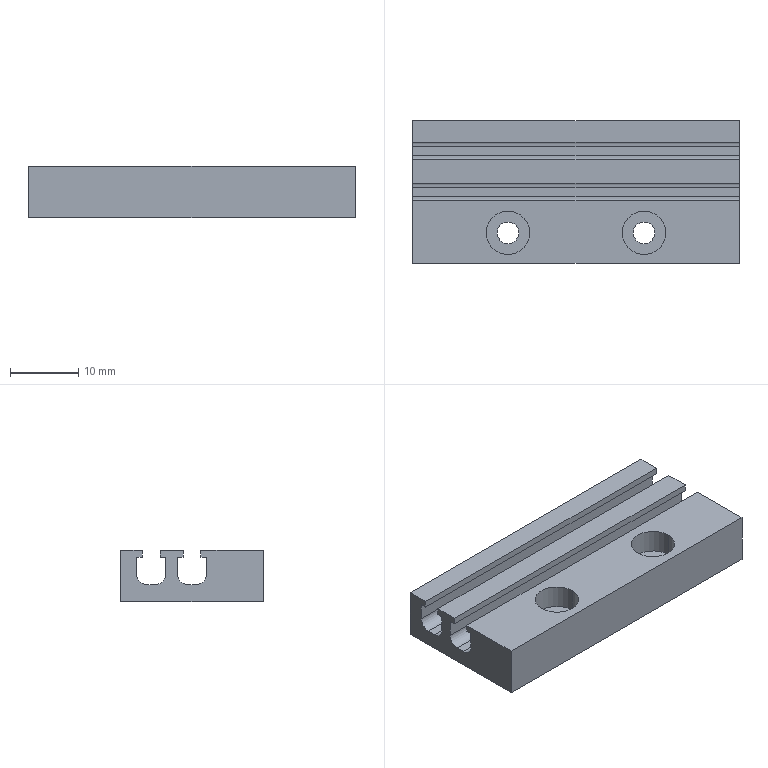Part | NX | 1 solid | 36 faces | box 48 x 21 x 7.5 mm | volume 5462 mm3 | plane 24 | cylinder 12 | commonest cylinder face diameters 3 x4 3.2 x4 6.4 x4
STEP:
#1=CARTESIAN_POINT('',(126.,-1.,-7.5));
#2=VERTEX_POINT('',#1);
#3=CARTESIAN_POINT('',(126.,-1.,0.));
#4=VERTEX_POINT('',#3);
#5=CARTESIAN_POINT('',(126.,-1.,0.));
#6=DIRECTION('',(0.,0.,1.));
#7=VECTOR('',#6,1000.);
#8=LINE('',#5,#7);
#9=EDGE_CURVE('',#2,#4,#8,.T.);
#10=ORIENTED_EDGE('',*,*,#9,.F.);
#11=CARTESIAN_POINT('',(126.,20.,-7.5));
#12=VERTEX_POINT('',#11);
#13=CARTESIAN_POINT('',(126.,0.,-7.5));
#14=DIRECTION('',(0.,1.,0.));
#15=VECTOR('',#14,1000.);
#16=LINE('',#13,#15);
#17=EDGE_CURVE('',#2,#12,#16,.T.);
#18=ORIENTED_EDGE('',*,*,#17,.T.);
#19=CARTESIAN_POINT('',(126.,20.,0.));
#20=VERTEX_POINT('',#19);
#21=CARTESIAN_POINT('',(126.,20.,0.));
#22=DIRECTION('',(0.,0.,1.));
#23=VECTOR('',#22,1000.);
#24=LINE('',#21,#23);
#25=EDGE_CURVE('',#12,#20,#24,.T.);
#26=ORIENTED_EDGE('',*,*,#25,.T.);
#27=CARTESIAN_POINT('',(126.,16.8,0.));
#28=VERTEX_POINT('',#27);
#29=CARTESIAN_POINT('',(126.,0.,0.));
#30=DIRECTION('',(0.,-1.,0.));
#31=VECTOR('',#30,1000.);
#32=LINE('',#29,#31);
#33=EDGE_CURVE('',#20,#28,#32,.T.);
#34=ORIENTED_EDGE('',*,*,#33,.T.);
#35=CARTESIAN_POINT('',(126.,16.8,-1.));
#36=VERTEX_POINT('',#35);
#37=CARTESIAN_POINT('',(126.,16.8,0.));
#38=DIRECTION('',(0.,0.,-1.));
#39=VECTOR('',#38,1000.);
#40=LINE('',#37,#39);
#41=EDGE_CURVE('',#28,#36,#40,.T.);
#42=ORIENTED_EDGE('',*,*,#41,.T.);
#43=CARTESIAN_POINT('',(126.,17.65,-1.));
#44=VERTEX_POINT('',#43);
#45=CARTESIAN_POINT('',(126.,0.,-1.));
#46=DIRECTION('',(0.,1.,0.));
#47=VECTOR('',#46,1000.);
#48=LINE('',#45,#47);
#49=EDGE_CURVE('',#36,#44,#48,.T.);
#50=ORIENTED_EDGE('',*,*,#49,.T.);
#51=CARTESIAN_POINT('',(126.,17.65,-3.5));
#52=VERTEX_POINT('',#51);
#53=CARTESIAN_POINT('',(126.,17.65,0.));
#54=DIRECTION('',(0.,0.,-1.));
#55=VECTOR('',#54,1000.);
#56=LINE('',#53,#55);
#57=EDGE_CURVE('',#44,#52,#56,.T.);
#58=ORIENTED_EDGE('',*,*,#57,.T.);
#59=CARTESIAN_POINT('',(126.,16.15,-5.));
#60=VERTEX_POINT('',#59);
#61=CARTESIAN_POINT('',(126.,16.15,-3.5));
#62=DIRECTION('',(1.,0.,0.));
#63=DIRECTION('',(0.,0.,-1.));
#64=AXIS2_PLACEMENT_3D('',#61,#62,#63);
#65=CIRCLE('',#64,1.5);
#66=EDGE_CURVE('',#60,#52,#65,.T.);
#67=ORIENTED_EDGE('',*,*,#66,.F.);
#68=CARTESIAN_POINT('',(126.,14.85,-5.));
#69=VERTEX_POINT('',#68);
#70=CARTESIAN_POINT('',(126.,0.,-5.));
#71=DIRECTION('',(0.,-1.,0.));
#72=VECTOR('',#71,1000.);
#73=LINE('',#70,#72);
#74=EDGE_CURVE('',#60,#69,#73,.T.);
#75=ORIENTED_EDGE('',*,*,#74,.T.);
#76=CARTESIAN_POINT('',(126.,13.35,-3.5));
#77=VERTEX_POINT('',#76);
#78=CARTESIAN_POINT('',(126.,14.85,-3.5));
#79=DIRECTION('',(1.,0.,0.));
#80=DIRECTION('',(0.,0.,-1.));
#81=AXIS2_PLACEMENT_3D('',#78,#79,#80);
#82=CIRCLE('',#81,1.5);
#83=EDGE_CURVE('',#77,#69,#82,.T.);
#84=ORIENTED_EDGE('',*,*,#83,.F.);
#85=CARTESIAN_POINT('',(126.,13.35,-1.));
#86=VERTEX_POINT('',#85);
#87=CARTESIAN_POINT('',(126.,13.35,0.));
#88=DIRECTION('',(0.,0.,1.));
#89=VECTOR('',#88,1000.);
#90=LINE('',#87,#89);
#91=EDGE_CURVE('',#77,#86,#90,.T.);
#92=ORIENTED_EDGE('',*,*,#91,.T.);
#93=CARTESIAN_POINT('',(126.,14.2,-1.));
#94=VERTEX_POINT('',#93);
#95=CARTESIAN_POINT('',(126.,0.,-1.));
#96=DIRECTION('',(0.,1.,0.));
#97=VECTOR('',#96,1000.);
#98=LINE('',#95,#97);
#99=EDGE_CURVE('',#86,#94,#98,.T.);
#100=ORIENTED_EDGE('',*,*,#99,.T.);
#101=CARTESIAN_POINT('',(126.,14.2,0.));
#102=VERTEX_POINT('',#101);
#103=CARTESIAN_POINT('',(126.,14.2,0.));
#104=DIRECTION('',(0.,0.,1.));
#105=VECTOR('',#104,1000.);
#106=LINE('',#103,#105);
#107=EDGE_CURVE('',#94,#102,#106,.T.);
#108=ORIENTED_EDGE('',*,*,#107,.T.);
#109=CARTESIAN_POINT('',(126.,10.8,0.));
#110=VERTEX_POINT('',#109);
#111=CARTESIAN_POINT('',(126.,0.,0.));
#112=DIRECTION('',(0.,-1.,0.));
#113=VECTOR('',#112,1000.);
#114=LINE('',#111,#113);
#115=EDGE_CURVE('',#102,#110,#114,.T.);
#116=ORIENTED_EDGE('',*,*,#115,.T.);
#117=CARTESIAN_POINT('',(126.,10.8,-1.));
#118=VERTEX_POINT('',#117);
#119=CARTESIAN_POINT('',(126.,10.8,0.));
#120=DIRECTION('',(0.,0.,-1.));
#121=VECTOR('',#120,1000.);
#122=LINE('',#119,#121);
#123=EDGE_CURVE('',#110,#118,#122,.T.);
#124=ORIENTED_EDGE('',*,*,#123,.T.);
#125=CARTESIAN_POINT('',(126.,11.65,-1.));
#126=VERTEX_POINT('',#125);
#127=CARTESIAN_POINT('',(126.,0.,-1.));
#128=DIRECTION('',(0.,1.,0.));
#129=VECTOR('',#128,1000.);
#130=LINE('',#127,#129);
#131=EDGE_CURVE('',#118,#126,#130,.T.);
#132=ORIENTED_EDGE('',*,*,#131,.T.);
#133=CARTESIAN_POINT('',(126.,11.65,-3.5));
#134=VERTEX_POINT('',#133);
#135=CARTESIAN_POINT('',(126.,11.65,0.));
#136=DIRECTION('',(0.,0.,-1.));
#137=VECTOR('',#136,1000.);
#138=LINE('',#135,#137);
#139=EDGE_CURVE('',#126,#134,#138,.T.);
#140=ORIENTED_EDGE('',*,*,#139,.T.);
#141=CARTESIAN_POINT('',(126.,10.15,-5.));
#142=VERTEX_POINT('',#141);
#143=CARTESIAN_POINT('',(126.,10.15,-3.5));
#144=DIRECTION('',(1.,0.,0.));
#145=DIRECTION('',(0.,0.,-1.));
#146=AXIS2_PLACEMENT_3D('',#143,#144,#145);
#147=CIRCLE('',#146,1.5);
#148=EDGE_CURVE('',#142,#134,#147,.T.);
#149=ORIENTED_EDGE('',*,*,#148,.F.);
#150=CARTESIAN_POINT('',(126.,8.85,-5.));
#151=VERTEX_POINT('',#150);
#152=CARTESIAN_POINT('',(126.,0.,-5.));
#153=DIRECTION('',(0.,-1.,0.));
#154=VECTOR('',#153,1000.);
#155=LINE('',#152,#154);
#156=EDGE_CURVE('',#142,#151,#155,.T.);
#157=ORIENTED_EDGE('',*,*,#156,.T.);
#158=CARTESIAN_POINT('',(126.,7.35,-3.5));
#159=VERTEX_POINT('',#158);
#160=CARTESIAN_POINT('',(126.,8.85,-3.5));
#161=DIRECTION('',(1.,0.,0.));
#162=DIRECTION('',(0.,0.,-1.));
#163=AXIS2_PLACEMENT_3D('',#160,#161,#162);
#164=CIRCLE('',#163,1.5);
#165=EDGE_CURVE('',#159,#151,#164,.T.);
#166=ORIENTED_EDGE('',*,*,#165,.F.);
#167=CARTESIAN_POINT('',(126.,7.35,-1.));
#168=VERTEX_POINT('',#167);
#169=CARTESIAN_POINT('',(126.,7.35,0.));
#170=DIRECTION('',(0.,0.,1.));
#171=VECTOR('',#170,1000.);
#172=LINE('',#169,#171);
#173=EDGE_CURVE('',#159,#168,#172,.T.);
#174=ORIENTED_EDGE('',*,*,#173,.T.);
#175=CARTESIAN_POINT('',(126.,8.2,-1.));
#176=VERTEX_POINT('',#175);
#177=CARTESIAN_POINT('',(126.,0.,-1.));
#178=DIRECTION('',(0.,1.,0.));
#179=VECTOR('',#178,1000.);
#180=LINE('',#177,#179);
#181=EDGE_CURVE('',#168,#176,#180,.T.);
#182=ORIENTED_EDGE('',*,*,#181,.T.);
#183=CARTESIAN_POINT('',(126.,8.2,0.));
#184=VERTEX_POINT('',#183);
#185=CARTESIAN_POINT('',(126.,8.2,0.));
#186=DIRECTION('',(0.,0.,1.));
#187=VECTOR('',#186,1000.);
#188=LINE('',#185,#187);
#189=EDGE_CURVE('',#176,#184,#188,.T.);
#190=ORIENTED_EDGE('',*,*,#189,.T.);
#191=CARTESIAN_POINT('',(126.,0.,0.));
#192=DIRECTION('',(0.,-1.,0.));
#193=VECTOR('',#192,1000.);
#194=LINE('',#191,#193);
#195=EDGE_CURVE('',#184,#4,#194,.T.);
#196=ORIENTED_EDGE('',*,*,#195,.T.);
#197=EDGE_LOOP('',(#10,#18,#26,#34,#42,#50,#58,#67,#75,#84,#92,#100,#108,#116,#124,#132,#140,#149,#157,#166,#174,#182,#190,#196));
#198=FACE_BOUND('',#197,.T.);
#199=CARTESIAN_POINT('',(126.,0.,0.));
#200=DIRECTION('',(1.,0.,0.));
#201=DIRECTION('',(0.,1.,0.));
#202=AXIS2_PLACEMENT_3D('',#199,#200,#201);
#203=PLANE('',#202);
#204=ADVANCED_FACE('',(#198),#203,.T.);
#205=CARTESIAN_POINT('',(78.,20.,0.));
#206=VERTEX_POINT('',#205);
#207=CARTESIAN_POINT('',(0.,20.,0.));
#208=DIRECTION('',(1.,0.,0.));
#209=VECTOR('',#208,1000.);
#210=LINE('',#207,#209);
#211=EDGE_CURVE('',#206,#20,#210,.T.);
#212=ORIENTED_EDGE('',*,*,#211,.F.);
#213=CARTESIAN_POINT('',(78.,16.8,0.));
#214=VERTEX_POINT('',#213);
#215=CARTESIAN_POINT('',(78.,0.,0.));
#216=DIRECTION('',(0.,-1.,0.));
#217=VECTOR('',#216,1000.);
#218=LINE('',#215,#217);
#219=EDGE_CURVE('',#206,#214,#218,.T.);
#220=ORIENTED_EDGE('',*,*,#219,.T.);
#221=CARTESIAN_POINT('',(0.,16.8,0.));
#222=DIRECTION('',(-1.,0.,0.));
#223=VECTOR('',#222,1000.);
#224=LINE('',#221,#223);
#225=EDGE_CURVE('',#28,#214,#224,.T.);
#226=ORIENTED_EDGE('',*,*,#225,.F.);
#227=ORIENTED_EDGE('',*,*,#33,.F.);
#228=EDGE_LOOP('',(#212,#220,#226,#227));
#229=FACE_BOUND('',#228,.T.);
#230=CARTESIAN_POINT('',(122.,19.,0.));
#231=DIRECTION('',(0.,0.,-1.));
#232=DIRECTION('',(0.,-1.,0.));
#233=AXIS2_PLACEMENT_3D('',#230,#231,#232);
#234=PLANE('',#233);
#235=ADVANCED_FACE('',(#229),#234,.F.);
#236=CARTESIAN_POINT('',(78.,20.,-7.5));
#237=VERTEX_POINT('',#236);
#238=CARTESIAN_POINT('',(0.,20.,-7.5));
#239=DIRECTION('',(-1.,0.,0.));
#240=VECTOR('',#239,1000.);
#241=LINE('',#238,#240);
#242=EDGE_CURVE('',#12,#237,#241,.T.);
#243=ORIENTED_EDGE('',*,*,#242,.T.);
#244=CARTESIAN_POINT('',(78.,20.,0.));
#245=DIRECTION('',(0.,0.,1.));
#246=VECTOR('',#245,1000.);
#247=LINE('',#244,#246);
#248=EDGE_CURVE('',#237,#206,#247,.T.);
#249=ORIENTED_EDGE('',*,*,#248,.T.);
#250=ORIENTED_EDGE('',*,*,#211,.T.);
#251=ORIENTED_EDGE('',*,*,#25,.F.);
#252=EDGE_LOOP('',(#243,#249,#250,#251));
#253=FACE_BOUND('',#252,.T.);
#254=CARTESIAN_POINT('',(122.,20.,-7.5));
#255=DIRECTION('',(0.,-1.,0.));
#256=DIRECTION('',(0.,0.,-1.));
#257=AXIS2_PLACEMENT_3D('',#254,#255,#256);
#258=PLANE('',#257);
#259=ADVANCED_FACE('',(#253),#258,.F.);
#260=CARTESIAN_POINT('',(78.,-1.,0.));
#261=VERTEX_POINT('',#260);
#262=CARTESIAN_POINT('',(0.,-1.,0.));
#263=DIRECTION('',(1.,0.,0.));
#264=VECTOR('',#263,1000.);
#265=LINE('',#262,#264);
#266=EDGE_CURVE('',#261,#4,#265,.T.);
#267=ORIENTED_EDGE('',*,*,#266,.T.);
#268=ORIENTED_EDGE('',*,*,#195,.F.);
#269=CARTESIAN_POINT('',(78.,8.2,0.));
#270=VERTEX_POINT('',#269);
#271=CARTESIAN_POINT('',(0.,8.2,0.));
#272=DIRECTION('',(1.,0.,0.));
#273=VECTOR('',#272,1000.);
#274=LINE('',#271,#273);
#275=EDGE_CURVE('',#270,#184,#274,.T.);
#276=ORIENTED_EDGE('',*,*,#275,.F.);
#277=CARTESIAN_POINT('',(78.,0.,0.));
#278=DIRECTION('',(0.,1.,0.));
#279=VECTOR('',#278,1000.);
#280=LINE('',#277,#279);
#281=EDGE_CURVE('',#261,#270,#280,.T.);
#282=ORIENTED_EDGE('',*,*,#281,.F.);
#283=EDGE_LOOP('',(#267,#268,#276,#282));
#284=FACE_BOUND('',#283,.T.);
#285=CARTESIAN_POINT('',(108.8,3.5,0.));
#286=VERTEX_POINT('',#285);
#287=CARTESIAN_POINT('',(115.2,3.5,0.));
#288=VERTEX_POINT('',#287);
#289=CARTESIAN_POINT('',(112.,3.5,0.));
#290=DIRECTION('',(0.,0.,-1.));
#291=DIRECTION('',(1.,0.,0.));
#292=AXIS2_PLACEMENT_3D('',#289,#290,#291);
#293=CIRCLE('',#292,3.2);
#294=EDGE_CURVE('',#286,#288,#293,.T.);
#295=ORIENTED_EDGE('',*,*,#294,.T.);
#296=CARTESIAN_POINT('',(112.,3.5,0.));
#297=DIRECTION('',(0.,0.,-1.));
#298=DIRECTION('',(1.,0.,0.));
#299=AXIS2_PLACEMENT_3D('',#296,#297,#298);
#300=CIRCLE('',#299,3.2);
#301=EDGE_CURVE('',#288,#286,#300,.T.);
#302=ORIENTED_EDGE('',*,*,#301,.T.);
#303=EDGE_LOOP('',(#295,#302));
#304=FACE_BOUND('',#303,.T.);
#305=CARTESIAN_POINT('',(95.2,3.5,0.));
#306=VERTEX_POINT('',#305);
#307=CARTESIAN_POINT('',(88.8,3.5,0.));
#308=VERTEX_POINT('',#307);
#309=CARTESIAN_POINT('',(92.,3.5,0.));
#310=DIRECTION('',(0.,0.,-1.));
#311=DIRECTION('',(1.,0.,0.));
#312=AXIS2_PLACEMENT_3D('',#309,#310,#311);
#313=CIRCLE('',#312,3.2);
#314=EDGE_CURVE('',#306,#308,#313,.T.);
#315=ORIENTED_EDGE('',*,*,#314,.T.);
#316=CARTESIAN_POINT('',(92.,3.5,0.));
#317=DIRECTION('',(0.,0.,-1.));
#318=DIRECTION('',(1.,0.,0.));
#319=AXIS2_PLACEMENT_3D('',#316,#317,#318);
#320=CIRCLE('',#319,3.2);
#321=EDGE_CURVE('',#308,#306,#320,.T.);
#322=ORIENTED_EDGE('',*,*,#321,.T.);
#323=EDGE_LOOP('',(#315,#322));
#324=FACE_BOUND('',#323,.T.);
#325=CARTESIAN_POINT('',(122.,8.2,0.));
#326=DIRECTION('',(0.,0.,-1.));
#327=DIRECTION('',(0.,-1.,0.));
#328=AXIS2_PLACEMENT_3D('',#325,#326,#327);
#329=PLANE('',#328);
#330=ADVANCED_FACE('',(#284,#304,#324),#329,.F.);
#331=ORIENTED_EDGE('',*,*,#314,.F.);
#332=CARTESIAN_POINT('',(95.2,3.5,-3.5));
#333=VERTEX_POINT('',#332);
#334=CARTESIAN_POINT('',(95.2,3.5,-8.662));
#335=DIRECTION('',(0.,0.,1.));
#336=VECTOR('',#335,1000.);
#337=LINE('',#334,#336);
#338=EDGE_CURVE('',#333,#306,#337,.T.);
#339=ORIENTED_EDGE('',*,*,#338,.F.);
#340=CARTESIAN_POINT('',(88.8,3.5,-3.5));
#341=VERTEX_POINT('',#340);
#342=CARTESIAN_POINT('',(92.,3.5,-3.5));
#343=DIRECTION('',(0.,0.,1.));
#344=DIRECTION('',(1.,0.,0.));
#345=AXIS2_PLACEMENT_3D('',#342,#343,#344);
#346=CIRCLE('',#345,3.2);
#347=EDGE_CURVE('',#341,#333,#346,.T.);
#348=ORIENTED_EDGE('',*,*,#347,.F.);
#349=CARTESIAN_POINT('',(88.8,3.5,-8.662));
#350=DIRECTION('',(0.,0.,1.));
#351=VECTOR('',#350,1000.);
#352=LINE('',#349,#351);
#353=EDGE_CURVE('',#341,#308,#352,.T.);
#354=ORIENTED_EDGE('',*,*,#353,.T.);
#355=EDGE_LOOP('',(#331,#339,#348,#354));
#356=FACE_BOUND('',#355,.T.);
#357=CARTESIAN_POINT('',(92.,3.5,-8.662));
#358=DIRECTION('',(0.,0.,1.));
#359=DIRECTION('',(1.,0.,0.));
#360=AXIS2_PLACEMENT_3D('',#357,#358,#359);
#361=CYLINDRICAL_SURFACE('',#360,3.2);
#362=ADVANCED_FACE('',(#356),#361,.F.);
#363=ORIENTED_EDGE('',*,*,#17,.F.);
#364=CARTESIAN_POINT('',(78.,-1.,-7.5));
#365=VERTEX_POINT('',#364);
#366=CARTESIAN_POINT('',(0.,-1.,-7.5));
#367=DIRECTION('',(-1.,0.,0.));
#368=VECTOR('',#367,1000.);
#369=LINE('',#366,#368);
#370=EDGE_CURVE('',#2,#365,#369,.T.);
#371=ORIENTED_EDGE('',*,*,#370,.T.);
#372=CARTESIAN_POINT('',(78.,0.,-7.5));
#373=DIRECTION('',(0.,-1.,0.));
#374=VECTOR('',#373,1000.);
#375=LINE('',#372,#374);
#376=EDGE_CURVE('',#237,#365,#375,.T.);
#377=ORIENTED_EDGE('',*,*,#376,.F.);
#378=ORIENTED_EDGE('',*,*,#242,.F.);
#379=EDGE_LOOP('',(#363,#371,#377,#378));
#380=FACE_BOUND('',#379,.T.);
#381=CARTESIAN_POINT('',(113.6,3.5,-7.5));
#382=VERTEX_POINT('',#381);
#383=CARTESIAN_POINT('',(110.4,3.5,-7.5));
#384=VERTEX_POINT('',#383);
#385=CARTESIAN_POINT('',(112.,3.5,-7.5));
#386=DIRECTION('',(0.,0.,-1.));
#387=DIRECTION('',(1.,0.,0.));
#388=AXIS2_PLACEMENT_3D('',#385,#386,#387);
#389=CIRCLE('',#388,1.6);
#390=EDGE_CURVE('',#382,#384,#389,.T.);
#391=ORIENTED_EDGE('',*,*,#390,.F.);
#392=CARTESIAN_POINT('',(112.,3.5,-7.5));
#393=DIRECTION('',(0.,0.,-1.));
#394=DIRECTION('',(1.,0.,0.));
#395=AXIS2_PLACEMENT_3D('',#392,#393,#394);
#396=CIRCLE('',#395,1.6);
#397=EDGE_CURVE('',#384,#382,#396,.T.);
#398=ORIENTED_EDGE('',*,*,#397,.F.);
#399=EDGE_LOOP('',(#391,#398));
#400=FACE_BOUND('',#399,.T.);
#401=CARTESIAN_POINT('',(90.4,3.5,-7.5));
#402=VERTEX_POINT('',#401);
#403=CARTESIAN_POINT('',(93.6,3.5,-7.5));
#404=VERTEX_POINT('',#403);
#405=CARTESIAN_POINT('',(92.,3.5,-7.5));
#406=DIRECTION('',(0.,0.,-1.));
#407=DIRECTION('',(1.,0.,0.));
#408=AXIS2_PLACEMENT_3D('',#405,#406,#407);
#409=CIRCLE('',#408,1.6);
#410=EDGE_CURVE('',#402,#404,#409,.T.);
#411=ORIENTED_EDGE('',*,*,#410,.F.);
#412=CARTESIAN_POINT('',(92.,3.5,-7.5));
#413=DIRECTION('',(0.,0.,-1.));
#414=DIRECTION('',(1.,0.,0.));
#415=AXIS2_PLACEMENT_3D('',#412,#413,#414);
#416=CIRCLE('',#415,1.6);
#417=EDGE_CURVE('',#404,#402,#416,.T.);
#418=ORIENTED_EDGE('',*,*,#417,.F.);
#419=EDGE_LOOP('',(#411,#418));
#420=FACE_BOUND('',#419,.T.);
#421=CARTESIAN_POINT('',(122.,0.,-7.5));
#422=DIRECTION('',(0.,0.,1.));
#423=DIRECTION('',(1.,0.,0.));
#424=AXIS2_PLACEMENT_3D('',#421,#422,#423);
#425=PLANE('',#424);
#426=ADVANCED_FACE('',(#380,#400,#420),#425,.F.);
#427=CARTESIAN_POINT('',(78.,8.2,-1.));
#428=VERTEX_POINT('',#427);
#429=CARTESIAN_POINT('',(0.,8.2,-1.));
#430=DIRECTION('',(1.,0.,0.));
#431=VECTOR('',#430,1000.);
#432=LINE('',#429,#431);
#433=EDGE_CURVE('',#428,#176,#432,.T.);
#434=ORIENTED_EDGE('',*,*,#433,.F.);
#435=CARTESIAN_POINT('',(78.,8.2,0.));
#436=DIRECTION('',(0.,0.,1.));
#437=VECTOR('',#436,1000.);
#438=LINE('',#435,#437);
#439=EDGE_CURVE('',#428,#270,#438,.T.);
#440=ORIENTED_EDGE('',*,*,#439,.T.);
#441=ORIENTED_EDGE('',*,*,#275,.T.);
#442=ORIENTED_EDGE('',*,*,#189,.F.);
#443=EDGE_LOOP('',(#434,#440,#441,#442));
#444=FACE_BOUND('',#443,.T.);
#445=CARTESIAN_POINT('',(122.,8.2,-1.));
#446=DIRECTION('',(0.,-1.,0.));
#447=DIRECTION('',(0.,0.,-1.));
#448=AXIS2_PLACEMENT_3D('',#445,#446,#447);
#449=PLANE('',#448);
#450=ADVANCED_FACE('',(#444),#449,.F.);
#451=CARTESIAN_POINT('',(78.,7.35,-1.));
#452=VERTEX_POINT('',#451);
#453=CARTESIAN_POINT('',(0.,7.35,-1.));
#454=DIRECTION('',(1.,0.,0.));
#455=VECTOR('',#454,1000.);
#456=LINE('',#453,#455);
#457=EDGE_CURVE('',#452,#168,#456,.T.);
#458=ORIENTED_EDGE('',*,*,#457,.F.);
#459=CARTESIAN_POINT('',(78.,0.,-1.));
#460=DIRECTION('',(0.,1.,0.));
#461=VECTOR('',#460,1000.);
#462=LINE('',#459,#461);
#463=EDGE_CURVE('',#452,#428,#462,.T.);
#464=ORIENTED_EDGE('',*,*,#463,.T.);
#465=ORIENTED_EDGE('',*,*,#433,.T.);
#466=ORIENTED_EDGE('',*,*,#181,.F.);
#467=EDGE_LOOP('',(#458,#464,#465,#466));
#468=FACE_BOUND('',#467,.T.);
#469=CARTESIAN_POINT('',(122.,7.35,-1.));
#470=DIRECTION('',(0.,0.,1.));
#471=DIRECTION('',(1.,0.,0.));
#472=AXIS2_PLACEMENT_3D('',#469,#470,#471);
#473=PLANE('',#472);
#474=ADVANCED_FACE('',(#468),#473,.F.);
#475=CARTESIAN_POINT('',(78.,7.35,-3.5));
#476=VERTEX_POINT('',#475);
#477=CARTESIAN_POINT('',(82.,7.35,-3.5));
#478=DIRECTION('',(1.,0.,0.));
#479=VECTOR('',#478,1000.);
#480=LINE('',#477,#479);
#481=EDGE_CURVE('',#476,#159,#480,.T.);
#482=ORIENTED_EDGE('',*,*,#481,.F.);
#483=CARTESIAN_POINT('',(78.,7.35,0.));
#484=DIRECTION('',(0.,0.,1.));
#485=VECTOR('',#484,1000.);
#486=LINE('',#483,#485);
#487=EDGE_CURVE('',#476,#452,#486,.T.);
#488=ORIENTED_EDGE('',*,*,#487,.T.);
#489=ORIENTED_EDGE('',*,*,#457,.T.);
#490=ORIENTED_EDGE('',*,*,#173,.F.);
#491=EDGE_LOOP('',(#482,#488,#489,#490));
#492=FACE_BOUND('',#491,.T.);
#493=CARTESIAN_POINT('',(122.,7.35,-3.5));
#494=DIRECTION('',(0.,-1.,0.));
#495=DIRECTION('',(0.,0.,-1.));
#496=AXIS2_PLACEMENT_3D('',#493,#494,#495);
#497=PLANE('',#496);
#498=ADVANCED_FACE('',(#492),#497,.F.);
#499=CARTESIAN_POINT('',(78.,8.85,-5.));
#500=VERTEX_POINT('',#499);
#501=CARTESIAN_POINT('',(122.,8.85,-5.));
#502=DIRECTION('',(-1.,0.,0.));
#503=VECTOR('',#502,1000.);
#504=LINE('',#501,#503);
#505=EDGE_CURVE('',#151,#500,#504,.T.);
#506=ORIENTED_EDGE('',*,*,#505,.T.);
#507=CARTESIAN_POINT('',(78.,8.85,-3.5));
#508=DIRECTION('',(1.,0.,0.));
#509=DIRECTION('',(0.,0.,-1.));
#510=AXIS2_PLACEMENT_3D('',#507,#508,#509);
#511=CIRCLE('',#510,1.5);
#512=EDGE_CURVE('',#476,#500,#511,.T.);
#513=ORIENTED_EDGE('',*,*,#512,.F.);
#514=ORIENTED_EDGE('',*,*,#481,.T.);
#515=ORIENTED_EDGE('',*,*,#165,.T.);
#516=EDGE_LOOP('',(#506,#513,#514,#515));
#517=FACE_BOUND('',#516,.T.);
#518=CARTESIAN_POINT('',(122.,8.85,-3.5));
#519=DIRECTION('',(-1.,0.,0.));
#520=DIRECTION('',(0.,0.,-1.));
#521=AXIS2_PLACEMENT_3D('',#518,#519,#520);
#522=CYLINDRICAL_SURFACE('',#521,1.5);
#523=ADVANCED_FACE('',(#517),#522,.F.);
#524=CARTESIAN_POINT('',(78.,10.15,-5.));
#525=VERTEX_POINT('',#524);
#526=CARTESIAN_POINT('',(122.,10.15,-5.));
#527=DIRECTION('',(-1.,0.,0.));
#528=VECTOR('',#527,1000.);
#529=LINE('',#526,#528);
#530=EDGE_CURVE('',#142,#525,#529,.T.);
#531=ORIENTED_EDGE('',*,*,#530,.T.);
#532=CARTESIAN_POINT('',(78.,0.,-5.));
#533=DIRECTION('',(0.,-1.,0.));
#534=VECTOR('',#533,1000.);
#535=LINE('',#532,#534);
#536=EDGE_CURVE('',#525,#500,#535,.T.);
#537=ORIENTED_EDGE('',*,*,#536,.T.);
#538=ORIENTED_EDGE('',*,*,#505,.F.);
#539=ORIENTED_EDGE('',*,*,#156,.F.);
#540=EDGE_LOOP('',(#531,#537,#538,#539));
#541=FACE_BOUND('',#540,.T.);
#542=CARTESIAN_POINT('',(122.,10.15,-5.));
#543=DIRECTION('',(0.,0.,-1.));
#544=DIRECTION('',(0.,-1.,0.));
#545=AXIS2_PLACEMENT_3D('',#542,#543,#544);
#546=PLANE('',#545);
#547=ADVANCED_FACE('',(#541),#546,.F.);
#548=CARTESIAN_POINT('',(78.,11.65,-3.5));
#549=VERTEX_POINT('',#548);
#550=CARTESIAN_POINT('',(122.,11.65,-3.5));
#551=DIRECTION('',(-1.,0.,0.));
#552=VECTOR('',#551,1000.);
#553=LINE('',#550,#552);
#554=EDGE_CURVE('',#134,#549,#553,.T.);
#555=ORIENTED_EDGE('',*,*,#554,.T.);
#556=CARTESIAN_POINT('',(78.,10.15,-3.5));
#557=DIRECTION('',(1.,0.,0.));
#558=DIRECTION('',(0.,0.,-1.));
#559=AXIS2_PLACEMENT_3D('',#556,#557,#558);
#560=CIRCLE('',#559,1.5);
#561=EDGE_CURVE('',#525,#549,#560,.T.);
#562=ORIENTED_EDGE('',*,*,#561,.F.);
#563=ORIENTED_EDGE('',*,*,#530,.F.);
#564=ORIENTED_EDGE('',*,*,#148,.T.);
#565=EDGE_LOOP('',(#555,#562,#563,#564));
#566=FACE_BOUND('',#565,.T.);
#567=CARTESIAN_POINT('',(122.,10.15,-3.5));
#568=DIRECTION('',(-1.,0.,0.));
#569=DIRECTION('',(0.,0.,-1.));
#570=AXIS2_PLACEMENT_3D('',#567,#568,#569);
#571=CYLINDRICAL_SURFACE('',#570,1.5);
#572=ADVANCED_FACE('',(#566),#571,.F.);
#573=CARTESIAN_POINT('',(78.,11.65,-1.));
#574=VERTEX_POINT('',#573);
#575=CARTESIAN_POINT('',(0.,11.65,-1.));
#576=DIRECTION('',(-1.,0.,0.));
#577=VECTOR('',#576,1000.);
#578=LINE('',#575,#577);
#579=EDGE_CURVE('',#126,#574,#578,.T.);
#580=ORIENTED_EDGE('',*,*,#579,.T.);
#581=CARTESIAN_POINT('',(78.,11.65,0.));
#582=DIRECTION('',(0.,0.,-1.));
#583=VECTOR('',#582,1000.);
#584=LINE('',#581,#583);
#585=EDGE_CURVE('',#574,#549,#584,.T.);
#586=ORIENTED_EDGE('',*,*,#585,.T.);
#587=ORIENTED_EDGE('',*,*,#554,.F.);
#588=ORIENTED_EDGE('',*,*,#139,.F.);
#589=EDGE_LOOP('',(#580,#586,#587,#588));
#590=FACE_BOUND('',#589,.T.);
#591=CARTESIAN_POINT('',(122.,11.65,-1.));
#592=DIRECTION('',(0.,1.,0.));
#593=DIRECTION('',(1.,0.,0.));
#594=AXIS2_PLACEMENT_3D('',#591,#592,#593);
#595=PLANE('',#594);
#596=ADVANCED_FACE('',(#590),#595,.F.);
#597=CARTESIAN_POINT('',(78.,10.8,-1.));
#598=VERTEX_POINT('',#597);
#599=CARTESIAN_POINT('',(0.,10.8,-1.));
#600=DIRECTION('',(-1.,0.,0.));
#601=VECTOR('',#600,1000.);
#602=LINE('',#599,#601);
#603=EDGE_CURVE('',#118,#598,#602,.T.);
#604=ORIENTED_EDGE('',*,*,#603,.T.);
#605=CARTESIAN_POINT('',(78.,0.,-1.));
#606=DIRECTION('',(0.,1.,0.));
#607=VECTOR('',#606,1000.);
#608=LINE('',#605,#607);
#609=EDGE_CURVE('',#598,#574,#608,.T.);
#610=ORIENTED_EDGE('',*,*,#609,.T.);
#611=ORIENTED_EDGE('',*,*,#579,.F.);
#612=ORIENTED_EDGE('',*,*,#131,.F.);
#613=EDGE_LOOP('',(#604,#610,#611,#612));
#614=FACE_BOUND('',#613,.T.);
#615=CARTESIAN_POINT('',(122.,10.8,-1.));
#616=DIRECTION('',(0.,0.,1.));
#617=DIRECTION('',(1.,0.,0.));
#618=AXIS2_PLACEMENT_3D('',#615,#616,#617);
#619=PLANE('',#618);
#620=ADVANCED_FACE('',(#614),#619,.F.);
#621=CARTESIAN_POINT('',(78.,10.8,0.));
#622=VERTEX_POINT('',#621);
#623=CARTESIAN_POINT('',(0.,10.8,0.));
#624=DIRECTION('',(-1.,0.,0.));
#625=VECTOR('',#624,1000.);
#626=LINE('',#623,#625);
#627=EDGE_CURVE('',#110,#622,#626,.T.);
#628=ORIENTED_EDGE('',*,*,#627,.T.);
#629=CARTESIAN_POINT('',(78.,10.8,0.));
#630=DIRECTION('',(0.,0.,-1.));
#631=VECTOR('',#630,1000.);
#632=LINE('',#629,#631);
#633=EDGE_CURVE('',#622,#598,#632,.T.);
#634=ORIENTED_EDGE('',*,*,#633,.T.);
#635=ORIENTED_EDGE('',*,*,#603,.F.);
#636=ORIENTED_EDGE('',*,*,#123,.F.);
#637=EDGE_LOOP('',(#628,#634,#635,#636));
#638=FACE_BOUND('',#637,.T.);
#639=CARTESIAN_POINT('',(122.,10.8,0.));
#640=DIRECTION('',(0.,1.,0.));
#641=DIRECTION('',(1.,0.,0.));
#642=AXIS2_PLACEMENT_3D('',#639,#640,#641);
#643=PLANE('',#642);
#644=ADVANCED_FACE('',(#638),#643,.F.);
#645=CARTESIAN_POINT('',(78.,14.2,0.));
#646=VERTEX_POINT('',#645);
#647=CARTESIAN_POINT('',(0.,14.2,0.));
#648=DIRECTION('',(1.,0.,0.));
#649=VECTOR('',#648,1000.);
#650=LINE('',#647,#649);
#651=EDGE_CURVE('',#646,#102,#650,.T.);
#652=ORIENTED_EDGE('',*,*,#651,.F.);
#653=CARTESIAN_POINT('',(78.,0.,0.));
#654=DIRECTION('',(0.,-1.,0.));
#655=VECTOR('',#654,1000.);
#656=LINE('',#653,#655);
#657=EDGE_CURVE('',#646,#622,#656,.T.);
#658=ORIENTED_EDGE('',*,*,#657,.T.);
#659=ORIENTED_EDGE('',*,*,#627,.F.);
#660=ORIENTED_EDGE('',*,*,#115,.F.);
#661=EDGE_LOOP('',(#652,#658,#659,#660));
#662=FACE_BOUND('',#661,.T.);
#663=CARTESIAN_POINT('',(122.,14.2,0.));
#664=DIRECTION('',(0.,0.,-1.));
#665=DIRECTION('',(0.,-1.,0.));
#666=AXIS2_PLACEMENT_3D('',#663,#664,#665);
#667=PLANE('',#666);
#668=ADVANCED_FACE('',(#662),#667,.F.);
#669=CARTESIAN_POINT('',(78.,14.2,-1.));
#670=VERTEX_POINT('',#669);
#671=CARTESIAN_POINT('',(0.,14.2,-1.));
#672=DIRECTION('',(-1.,0.,0.));
#673=VECTOR('',#672,1000.);
#674=LINE('',#671,#673);
#675=EDGE_CURVE('',#94,#670,#674,.T.);
#676=ORIENTED_EDGE('',*,*,#675,.T.);
#677=CARTESIAN_POINT('',(78.,14.2,0.));
#678=DIRECTION('',(0.,0.,1.));
#679=VECTOR('',#678,1000.);
#680=LINE('',#677,#679);
#681=EDGE_CURVE('',#670,#646,#680,.T.);
#682=ORIENTED_EDGE('',*,*,#681,.T.);
#683=ORIENTED_EDGE('',*,*,#651,.T.);
#684=ORIENTED_EDGE('',*,*,#107,.F.);
#685=EDGE_LOOP('',(#676,#682,#683,#684));
#686=FACE_BOUND('',#685,.T.);
#687=CARTESIAN_POINT('',(122.,14.2,-1.));
#688=DIRECTION('',(0.,-1.,0.));
#689=DIRECTION('',(0.,0.,-1.));
#690=AXIS2_PLACEMENT_3D('',#687,#688,#689);
#691=PLANE('',#690);
#692=ADVANCED_FACE('',(#686),#691,.F.);
#693=CARTESIAN_POINT('',(78.,13.35,-1.));
#694=VERTEX_POINT('',#693);
#695=CARTESIAN_POINT('',(0.,13.35,-1.));
#696=DIRECTION('',(1.,0.,0.));
#697=VECTOR('',#696,1000.);
#698=LINE('',#695,#697);
#699=EDGE_CURVE('',#694,#86,#698,.T.);
#700=ORIENTED_EDGE('',*,*,#699,.F.);
#701=CARTESIAN_POINT('',(78.,0.,-1.));
#702=DIRECTION('',(0.,1.,0.));
#703=VECTOR('',#702,1000.);
#704=LINE('',#701,#703);
#705=EDGE_CURVE('',#694,#670,#704,.T.);
#706=ORIENTED_EDGE('',*,*,#705,.T.);
#707=ORIENTED_EDGE('',*,*,#675,.F.);
#708=ORIENTED_EDGE('',*,*,#99,.F.);
#709=EDGE_LOOP('',(#700,#706,#707,#708));
#710=FACE_BOUND('',#709,.T.);
#711=CARTESIAN_POINT('',(122.,13.35,-1.));
#712=DIRECTION('',(0.,0.,1.));
#713=DIRECTION('',(1.,0.,0.));
#714=AXIS2_PLACEMENT_3D('',#711,#712,#713);
#715=PLANE('',#714);
#716=ADVANCED_FACE('',(#710),#715,.F.);
#717=CARTESIAN_POINT('',(78.,13.35,-3.5));
#718=VERTEX_POINT('',#717);
#719=CARTESIAN_POINT('',(82.,13.35,-3.5));
#720=DIRECTION('',(1.,0.,0.));
#721=VECTOR('',#720,1000.);
#722=LINE('',#719,#721);
#723=EDGE_CURVE('',#718,#77,#722,.T.);
#724=ORIENTED_EDGE('',*,*,#723,.F.);
#725=CARTESIAN_POINT('',(78.,13.35,0.));
#726=DIRECTION('',(0.,0.,1.));
#727=VECTOR('',#726,1000.);
#728=LINE('',#725,#727);
#729=EDGE_CURVE('',#718,#694,#728,.T.);
#730=ORIENTED_EDGE('',*,*,#729,.T.);
#731=ORIENTED_EDGE('',*,*,#699,.T.);
#732=ORIENTED_EDGE('',*,*,#91,.F.);
#733=EDGE_LOOP('',(#724,#730,#731,#732));
#734=FACE_BOUND('',#733,.T.);
#735=CARTESIAN_POINT('',(122.,13.35,-3.5));
#736=DIRECTION('',(0.,-1.,0.));
#737=DIRECTION('',(0.,0.,-1.));
#738=AXIS2_PLACEMENT_3D('',#735,#736,#737);
#739=PLANE('',#738);
#740=ADVANCED_FACE('',(#734),#739,.F.);
#741=CARTESIAN_POINT('',(78.,14.85,-5.));
#742=VERTEX_POINT('',#741);
#743=CARTESIAN_POINT('',(122.,14.85,-5.));
#744=DIRECTION('',(-1.,0.,0.));
#745=VECTOR('',#744,1000.);
#746=LINE('',#743,#745);
#747=EDGE_CURVE('',#69,#742,#746,.T.);
#748=ORIENTED_EDGE('',*,*,#747,.T.);
#749=CARTESIAN_POINT('',(78.,14.85,-3.5));
#750=DIRECTION('',(1.,0.,0.));
#751=DIRECTION('',(0.,0.,-1.));
#752=AXIS2_PLACEMENT_3D('',#749,#750,#751);
#753=CIRCLE('',#752,1.5);
#754=EDGE_CURVE('',#718,#742,#753,.T.);
#755=ORIENTED_EDGE('',*,*,#754,.F.);
#756=ORIENTED_EDGE('',*,*,#723,.T.);
#757=ORIENTED_EDGE('',*,*,#83,.T.);
#758=EDGE_LOOP('',(#748,#755,#756,#757));
#759=FACE_BOUND('',#758,.T.);
#760=CARTESIAN_POINT('',(122.,14.85,-3.5));
#761=DIRECTION('',(-1.,0.,0.));
#762=DIRECTION('',(0.,0.,-1.));
#763=AXIS2_PLACEMENT_3D('',#760,#761,#762);
#764=CYLINDRICAL_SURFACE('',#763,1.5);
#765=ADVANCED_FACE('',(#759),#764,.F.);
#766=CARTESIAN_POINT('',(78.,16.15,-5.));
#767=VERTEX_POINT('',#766);
#768=CARTESIAN_POINT('',(122.,16.15,-5.));
#769=DIRECTION('',(-1.,0.,0.));
#770=VECTOR('',#769,1000.);
#771=LINE('',#768,#770);
#772=EDGE_CURVE('',#60,#767,#771,.T.);
#773=ORIENTED_EDGE('',*,*,#772,.T.);
#774=CARTESIAN_POINT('',(78.,0.,-5.));
#775=DIRECTION('',(0.,-1.,0.));
#776=VECTOR('',#775,1000.);
#777=LINE('',#774,#776);
#778=EDGE_CURVE('',#767,#742,#777,.T.);
#779=ORIENTED_EDGE('',*,*,#778,.T.);
#780=ORIENTED_EDGE('',*,*,#747,.F.);
#781=ORIENTED_EDGE('',*,*,#74,.F.);
#782=EDGE_LOOP('',(#773,#779,#780,#781));
#783=FACE_BOUND('',#782,.T.);
#784=CARTESIAN_POINT('',(122.,16.15,-5.));
#785=DIRECTION('',(0.,0.,-1.));
#786=DIRECTION('',(0.,-1.,0.));
#787=AXIS2_PLACEMENT_3D('',#784,#785,#786);
#788=PLANE('',#787);
#789=ADVANCED_FACE('',(#783),#788,.F.);
#790=CARTESIAN_POINT('',(78.,17.65,-3.5));
#791=VERTEX_POINT('',#790);
#792=CARTESIAN_POINT('',(122.,17.65,-3.5));
#793=DIRECTION('',(-1.,0.,0.));
#794=VECTOR('',#793,1000.);
#795=LINE('',#792,#794);
#796=EDGE_CURVE('',#52,#791,#795,.T.);
#797=ORIENTED_EDGE('',*,*,#796,.T.);
#798=CARTESIAN_POINT('',(78.,16.15,-3.5));
#799=DIRECTION('',(1.,0.,0.));
#800=DIRECTION('',(0.,0.,-1.));
#801=AXIS2_PLACEMENT_3D('',#798,#799,#800);
#802=CIRCLE('',#801,1.5);
#803=EDGE_CURVE('',#767,#791,#802,.T.);
#804=ORIENTED_EDGE('',*,*,#803,.F.);
#805=ORIENTED_EDGE('',*,*,#772,.F.);
#806=ORIENTED_EDGE('',*,*,#66,.T.);
#807=EDGE_LOOP('',(#797,#804,#805,#806));
#808=FACE_BOUND('',#807,.T.);
#809=CARTESIAN_POINT('',(122.,16.15,-3.5));
#810=DIRECTION('',(-1.,0.,0.));
#811=DIRECTION('',(0.,0.,-1.));
#812=AXIS2_PLACEMENT_3D('',#809,#810,#811);
#813=CYLINDRICAL_SURFACE('',#812,1.5);
#814=ADVANCED_FACE('',(#808),#813,.F.);
#815=CARTESIAN_POINT('',(78.,17.65,-1.));
#816=VERTEX_POINT('',#815);
#817=CARTESIAN_POINT('',(0.,17.65,-1.));
#818=DIRECTION('',(-1.,0.,0.));
#819=VECTOR('',#818,1000.);
#820=LINE('',#817,#819);
#821=EDGE_CURVE('',#44,#816,#820,.T.);
#822=ORIENTED_EDGE('',*,*,#821,.T.);
#823=CARTESIAN_POINT('',(78.,17.65,0.));
#824=DIRECTION('',(0.,0.,-1.));
#825=VECTOR('',#824,1000.);
#826=LINE('',#823,#825);
#827=EDGE_CURVE('',#816,#791,#826,.T.);
#828=ORIENTED_EDGE('',*,*,#827,.T.);
#829=ORIENTED_EDGE('',*,*,#796,.F.);
#830=ORIENTED_EDGE('',*,*,#57,.F.);
#831=EDGE_LOOP('',(#822,#828,#829,#830));
#832=FACE_BOUND('',#831,.T.);
#833=CARTESIAN_POINT('',(122.,17.65,-1.));
#834=DIRECTION('',(0.,1.,0.));
#835=DIRECTION('',(1.,0.,0.));
#836=AXIS2_PLACEMENT_3D('',#833,#834,#835);
#837=PLANE('',#836);
#838=ADVANCED_FACE('',(#832),#837,.F.);
#839=CARTESIAN_POINT('',(78.,16.8,-1.));
#840=VERTEX_POINT('',#839);
#841=CARTESIAN_POINT('',(0.,16.8,-1.));
#842=DIRECTION('',(-1.,0.,0.));
#843=VECTOR('',#842,1000.);
#844=LINE('',#841,#843);
#845=EDGE_CURVE('',#36,#840,#844,.T.);
#846=ORIENTED_EDGE('',*,*,#845,.T.);
#847=CARTESIAN_POINT('',(78.,0.,-1.));
#848=DIRECTION('',(0.,1.,0.));
#849=VECTOR('',#848,1000.);
#850=LINE('',#847,#849);
#851=EDGE_CURVE('',#840,#816,#850,.T.);
#852=ORIENTED_EDGE('',*,*,#851,.T.);
#853=ORIENTED_EDGE('',*,*,#821,.F.);
#854=ORIENTED_EDGE('',*,*,#49,.F.);
#855=EDGE_LOOP('',(#846,#852,#853,#854));
#856=FACE_BOUND('',#855,.T.);
#857=CARTESIAN_POINT('',(122.,16.8,-1.));
#858=DIRECTION('',(0.,0.,1.));
#859=DIRECTION('',(1.,0.,0.));
#860=AXIS2_PLACEMENT_3D('',#857,#858,#859);
#861=PLANE('',#860);
#862=ADVANCED_FACE('',(#856),#861,.F.);
#863=ORIENTED_EDGE('',*,*,#225,.T.);
#864=CARTESIAN_POINT('',(78.,16.8,0.));
#865=DIRECTION('',(0.,0.,-1.));
#866=VECTOR('',#865,1000.);
#867=LINE('',#864,#866);
#868=EDGE_CURVE('',#214,#840,#867,.T.);
#869=ORIENTED_EDGE('',*,*,#868,.T.);
#870=ORIENTED_EDGE('',*,*,#845,.F.);
#871=ORIENTED_EDGE('',*,*,#41,.F.);
#872=EDGE_LOOP('',(#863,#869,#870,#871));
#873=FACE_BOUND('',#872,.T.);
#874=CARTESIAN_POINT('',(122.,16.8,0.));
#875=DIRECTION('',(0.,1.,0.));
#876=DIRECTION('',(1.,0.,0.));
#877=AXIS2_PLACEMENT_3D('',#874,#875,#876);
#878=PLANE('',#877);
#879=ADVANCED_FACE('',(#873),#878,.F.);
#880=ORIENTED_EDGE('',*,*,#248,.F.);
#881=ORIENTED_EDGE('',*,*,#376,.T.);
#882=CARTESIAN_POINT('',(78.,-1.,0.));
#883=DIRECTION('',(0.,0.,1.));
#884=VECTOR('',#883,1000.);
#885=LINE('',#882,#884);
#886=EDGE_CURVE('',#365,#261,#885,.T.);
#887=ORIENTED_EDGE('',*,*,#886,.T.);
#888=ORIENTED_EDGE('',*,*,#281,.T.);
#889=ORIENTED_EDGE('',*,*,#439,.F.);
#890=ORIENTED_EDGE('',*,*,#463,.F.);
#891=ORIENTED_EDGE('',*,*,#487,.F.);
#892=ORIENTED_EDGE('',*,*,#512,.T.);
#893=ORIENTED_EDGE('',*,*,#536,.F.);
#894=ORIENTED_EDGE('',*,*,#561,.T.);
#895=ORIENTED_EDGE('',*,*,#585,.F.);
#896=ORIENTED_EDGE('',*,*,#609,.F.);
#897=ORIENTED_EDGE('',*,*,#633,.F.);
#898=ORIENTED_EDGE('',*,*,#657,.F.);
#899=ORIENTED_EDGE('',*,*,#681,.F.);
#900=ORIENTED_EDGE('',*,*,#705,.F.);
#901=ORIENTED_EDGE('',*,*,#729,.F.);
#902=ORIENTED_EDGE('',*,*,#754,.T.);
#903=ORIENTED_EDGE('',*,*,#778,.F.);
#904=ORIENTED_EDGE('',*,*,#803,.T.);
#905=ORIENTED_EDGE('',*,*,#827,.F.);
#906=ORIENTED_EDGE('',*,*,#851,.F.);
#907=ORIENTED_EDGE('',*,*,#868,.F.);
#908=ORIENTED_EDGE('',*,*,#219,.F.);
#909=EDGE_LOOP('',(#880,#881,#887,#888,#889,#890,#891,#892,#893,#894,#895,#896,#897,#898,#899,#900,#901,#902,#903,#904,#905,#906,#907,#908));
#910=FACE_BOUND('',#909,.T.);
#911=CARTESIAN_POINT('',(78.,0.,0.));
#912=DIRECTION('',(1.,0.,0.));
#913=DIRECTION('',(0.,1.,0.));
#914=AXIS2_PLACEMENT_3D('',#911,#912,#913);
#915=PLANE('',#914);
#916=ADVANCED_FACE('',(#910),#915,.F.);
#917=ORIENTED_EDGE('',*,*,#9,.T.);
#918=ORIENTED_EDGE('',*,*,#266,.F.);
#919=ORIENTED_EDGE('',*,*,#886,.F.);
#920=ORIENTED_EDGE('',*,*,#370,.F.);
#921=EDGE_LOOP('',(#917,#918,#919,#920));
#922=FACE_BOUND('',#921,.T.);
#923=CARTESIAN_POINT('',(122.,-1.,0.));
#924=DIRECTION('',(0.,1.,0.));
#925=DIRECTION('',(1.,0.,0.));
#926=AXIS2_PLACEMENT_3D('',#923,#924,#925);
#927=PLANE('',#926);
#928=ADVANCED_FACE('',(#922),#927,.F.);
#929=ORIENTED_EDGE('',*,*,#294,.F.);
#930=CARTESIAN_POINT('',(108.8,3.5,-3.5));
#931=VERTEX_POINT('',#930);
#932=CARTESIAN_POINT('',(108.8,3.5,-8.662));
#933=DIRECTION('',(0.,0.,1.));
#934=VECTOR('',#933,1000.);
#935=LINE('',#932,#934);
#936=EDGE_CURVE('',#286,#931,#935,.F.);
#937=ORIENTED_EDGE('',*,*,#936,.T.);
#938=CARTESIAN_POINT('',(115.2,3.5,-3.5));
#939=VERTEX_POINT('',#938);
#940=CARTESIAN_POINT('',(112.,3.5,-3.5));
#941=DIRECTION('',(0.,0.,1.));
#942=DIRECTION('',(-1.,0.,0.));
#943=AXIS2_PLACEMENT_3D('',#940,#941,#942);
#944=CIRCLE('',#943,3.2);
#945=EDGE_CURVE('',#939,#931,#944,.T.);
#946=ORIENTED_EDGE('',*,*,#945,.F.);
#947=CARTESIAN_POINT('',(115.2,3.5,-8.662));
#948=DIRECTION('',(0.,0.,1.));
#949=VECTOR('',#948,1000.);
#950=LINE('',#947,#949);
#951=EDGE_CURVE('',#288,#939,#950,.F.);
#952=ORIENTED_EDGE('',*,*,#951,.F.);
#953=EDGE_LOOP('',(#929,#937,#946,#952));
#954=FACE_BOUND('',#953,.T.);
#955=CARTESIAN_POINT('',(112.,3.5,-8.662));
#956=DIRECTION('',(0.,0.,1.));
#957=DIRECTION('',(1.,0.,0.));
#958=AXIS2_PLACEMENT_3D('',#955,#956,#957);
#959=CYLINDRICAL_SURFACE('',#958,3.2);
#960=ADVANCED_FACE('',(#954),#959,.F.);
#961=CARTESIAN_POINT('',(92.,3.5,-3.5));
#962=DIRECTION('',(0.,0.,1.));
#963=DIRECTION('',(1.,0.,0.));
#964=AXIS2_PLACEMENT_3D('',#961,#962,#963);
#965=CIRCLE('',#964,3.2);
#966=EDGE_CURVE('',#333,#341,#965,.T.);
#967=ORIENTED_EDGE('',*,*,#966,.T.);
#968=ORIENTED_EDGE('',*,*,#347,.T.);
#969=EDGE_LOOP('',(#967,#968));
#970=FACE_BOUND('',#969,.T.);
#971=CARTESIAN_POINT('',(93.6,3.5,-3.5));
#972=VERTEX_POINT('',#971);
#973=CARTESIAN_POINT('',(90.4,3.5,-3.5));
#974=VERTEX_POINT('',#973);
#975=CARTESIAN_POINT('',(92.,3.5,-3.5));
#976=DIRECTION('',(0.,0.,-1.));
#977=DIRECTION('',(1.,0.,0.));
#978=AXIS2_PLACEMENT_3D('',#975,#976,#977);
#979=CIRCLE('',#978,1.6);
#980=EDGE_CURVE('',#972,#974,#979,.T.);
#981=ORIENTED_EDGE('',*,*,#980,.T.);
#982=CARTESIAN_POINT('',(92.,3.5,-3.5));
#983=DIRECTION('',(0.,0.,-1.));
#984=DIRECTION('',(1.,0.,0.));
#985=AXIS2_PLACEMENT_3D('',#982,#983,#984);
#986=CIRCLE('',#985,1.6);
#987=EDGE_CURVE('',#974,#972,#986,.T.);
#988=ORIENTED_EDGE('',*,*,#987,.T.);
#989=EDGE_LOOP('',(#981,#988));
#990=FACE_BOUND('',#989,.T.);
#991=CARTESIAN_POINT('',(92.,3.5,-3.5));
#992=DIRECTION('',(0.,0.,-1.));
#993=DIRECTION('',(0.,-1.,0.));
#994=AXIS2_PLACEMENT_3D('',#991,#992,#993);
#995=PLANE('',#994);
#996=ADVANCED_FACE('',(#970,#990),#995,.F.);
#997=CARTESIAN_POINT('',(112.,3.5,-3.5));
#998=DIRECTION('',(0.,0.,1.));
#999=DIRECTION('',(-1.,0.,0.));
#1000=AXIS2_PLACEMENT_3D('',#997,#998,#999);
#1001=CIRCLE('',#1000,3.2);
#1002=EDGE_CURVE('',#931,#939,#1001,.T.);
#1003=ORIENTED_EDGE('',*,*,#1002,.T.);
#1004=ORIENTED_EDGE('',*,*,#945,.T.);
#1005=EDGE_LOOP('',(#1003,#1004));
#1006=FACE_BOUND('',#1005,.T.);
#1007=CARTESIAN_POINT('',(110.4,3.5,-3.5));
#1008=VERTEX_POINT('',#1007);
#1009=CARTESIAN_POINT('',(113.6,3.5,-3.5));
#1010=VERTEX_POINT('',#1009);
#1011=CARTESIAN_POINT('',(112.,3.5,-3.5));
#1012=DIRECTION('',(0.,0.,-1.));
#1013=DIRECTION('',(1.,0.,0.));
#1014=AXIS2_PLACEMENT_3D('',#1011,#1012,#1013);
#1015=CIRCLE('',#1014,1.6);
#1016=EDGE_CURVE('',#1008,#1010,#1015,.T.);
#1017=ORIENTED_EDGE('',*,*,#1016,.T.);
#1018=CARTESIAN_POINT('',(112.,3.5,-3.5));
#1019=DIRECTION('',(0.,0.,-1.));
#1020=DIRECTION('',(1.,0.,0.));
#1021=AXIS2_PLACEMENT_3D('',#1018,#1019,#1020);
#1022=CIRCLE('',#1021,1.6);
#1023=EDGE_CURVE('',#1010,#1008,#1022,.T.);
#1024=ORIENTED_EDGE('',*,*,#1023,.T.);
#1025=EDGE_LOOP('',(#1017,#1024));
#1026=FACE_BOUND('',#1025,.T.);
#1027=CARTESIAN_POINT('',(112.,3.5,-3.5));
#1028=DIRECTION('',(0.,0.,-1.));
#1029=DIRECTION('',(0.,-1.,0.));
#1030=AXIS2_PLACEMENT_3D('',#1027,#1028,#1029);
#1031=PLANE('',#1030);
#1032=ADVANCED_FACE('',(#1006,#1026),#1031,.F.);
#1033=ORIENTED_EDGE('',*,*,#390,.T.);
#1034=CARTESIAN_POINT('',(110.4,3.5,-8.662));
#1035=DIRECTION('',(0.,0.,1.));
#1036=VECTOR('',#1035,1000.);
#1037=LINE('',#1034,#1036);
#1038=EDGE_CURVE('',#1008,#384,#1037,.F.);
#1039=ORIENTED_EDGE('',*,*,#1038,.F.);
#1040=ORIENTED_EDGE('',*,*,#1023,.F.);
#1041=CARTESIAN_POINT('',(113.6,3.5,-8.662));
#1042=DIRECTION('',(0.,0.,1.));
#1043=VECTOR('',#1042,1000.);
#1044=LINE('',#1041,#1043);
#1045=EDGE_CURVE('',#1010,#382,#1044,.F.);
#1046=ORIENTED_EDGE('',*,*,#1045,.T.);
#1047=EDGE_LOOP('',(#1033,#1039,#1040,#1046));
#1048=FACE_BOUND('',#1047,.T.);
#1049=CARTESIAN_POINT('',(112.,3.5,-8.662));
#1050=DIRECTION('',(0.,0.,1.));
#1051=DIRECTION('',(1.,0.,0.));
#1052=AXIS2_PLACEMENT_3D('',#1049,#1050,#1051);
#1053=CYLINDRICAL_SURFACE('',#1052,1.6);
#1054=ADVANCED_FACE('',(#1048),#1053,.F.);
#1055=ORIENTED_EDGE('',*,*,#980,.F.);
#1056=CARTESIAN_POINT('',(93.6,3.5,-8.662));
#1057=DIRECTION('',(0.,0.,1.));
#1058=VECTOR('',#1057,1000.);
#1059=LINE('',#1056,#1058);
#1060=EDGE_CURVE('',#404,#972,#1059,.T.);
#1061=ORIENTED_EDGE('',*,*,#1060,.F.);
#1062=ORIENTED_EDGE('',*,*,#417,.T.);
#1063=CARTESIAN_POINT('',(90.4,3.5,-8.662));
#1064=DIRECTION('',(0.,0.,1.));
#1065=VECTOR('',#1064,1000.);
#1066=LINE('',#1063,#1065);
#1067=EDGE_CURVE('',#402,#974,#1066,.T.);
#1068=ORIENTED_EDGE('',*,*,#1067,.T.);
#1069=EDGE_LOOP('',(#1055,#1061,#1062,#1068));
#1070=FACE_BOUND('',#1069,.T.);
#1071=CARTESIAN_POINT('',(92.,3.5,-8.662));
#1072=DIRECTION('',(0.,0.,1.));
#1073=DIRECTION('',(1.,0.,0.));
#1074=AXIS2_PLACEMENT_3D('',#1071,#1072,#1073);
#1075=CYLINDRICAL_SURFACE('',#1074,1.6);
#1076=ADVANCED_FACE('',(#1070),#1075,.F.);
#1077=ORIENTED_EDGE('',*,*,#1002,.F.);
#1078=ORIENTED_EDGE('',*,*,#936,.F.);
#1079=ORIENTED_EDGE('',*,*,#301,.F.);
#1080=ORIENTED_EDGE('',*,*,#951,.T.);
#1081=EDGE_LOOP('',(#1077,#1078,#1079,#1080));
#1082=FACE_BOUND('',#1081,.T.);
#1083=CARTESIAN_POINT('',(112.,3.5,-8.662));
#1084=DIRECTION('',(0.,0.,1.));
#1085=DIRECTION('',(1.,0.,0.));
#1086=AXIS2_PLACEMENT_3D('',#1083,#1084,#1085);
#1087=CYLINDRICAL_SURFACE('',#1086,3.2);
#1088=ADVANCED_FACE('',(#1082),#1087,.F.);
#1089=ORIENTED_EDGE('',*,*,#966,.F.);
#1090=ORIENTED_EDGE('',*,*,#338,.T.);
#1091=ORIENTED_EDGE('',*,*,#321,.F.);
#1092=ORIENTED_EDGE('',*,*,#353,.F.);
#1093=EDGE_LOOP('',(#1089,#1090,#1091,#1092));
#1094=FACE_BOUND('',#1093,.T.);
#1095=CARTESIAN_POINT('',(92.,3.5,-8.662));
#1096=DIRECTION('',(0.,0.,1.));
#1097=DIRECTION('',(1.,0.,0.));
#1098=AXIS2_PLACEMENT_3D('',#1095,#1096,#1097);
#1099=CYLINDRICAL_SURFACE('',#1098,3.2);
#1100=ADVANCED_FACE('',(#1094),#1099,.F.);
#1101=ORIENTED_EDGE('',*,*,#410,.T.);
#1102=ORIENTED_EDGE('',*,*,#1060,.T.);
#1103=ORIENTED_EDGE('',*,*,#987,.F.);
#1104=ORIENTED_EDGE('',*,*,#1067,.F.);
#1105=EDGE_LOOP('',(#1101,#1102,#1103,#1104));
#1106=FACE_BOUND('',#1105,.T.);
#1107=CARTESIAN_POINT('',(92.,3.5,-8.662));
#1108=DIRECTION('',(0.,0.,1.));
#1109=DIRECTION('',(1.,0.,0.));
#1110=AXIS2_PLACEMENT_3D('',#1107,#1108,#1109);
#1111=CYLINDRICAL_SURFACE('',#1110,1.6);
#1112=ADVANCED_FACE('',(#1106),#1111,.F.);
#1113=ORIENTED_EDGE('',*,*,#1016,.F.);
#1114=ORIENTED_EDGE('',*,*,#1038,.T.);
#1115=ORIENTED_EDGE('',*,*,#397,.T.);
#1116=ORIENTED_EDGE('',*,*,#1045,.F.);
#1117=EDGE_LOOP('',(#1113,#1114,#1115,#1116));
#1118=FACE_BOUND('',#1117,.T.);
#1119=CARTESIAN_POINT('',(112.,3.5,-8.662));
#1120=DIRECTION('',(0.,0.,1.));
#1121=DIRECTION('',(1.,0.,0.));
#1122=AXIS2_PLACEMENT_3D('',#1119,#1120,#1121);
#1123=CYLINDRICAL_SURFACE('',#1122,1.6);
#1124=ADVANCED_FACE('',(#1118),#1123,.F.);
#1125=CLOSED_SHELL('',(#204,#235,#259,#330,#362,#426,#450,#474,#498,#523,#547,#572,#596,#620,#644,#668,#692,#716,#740,#765,#789,#814,#838,#862,#879,#916,#928,#960,#996,#1032,#1054,#1076,#1088,#1100,#1112,#1124));
#1126=MANIFOLD_SOLID_BREP('',#1125);
#1127=(LENGTH_UNIT()NAMED_UNIT(*)SI_UNIT(.MILLI.,.METRE.));
#1128=UNCERTAINTY_MEASURE_WITH_UNIT(LENGTH_MEASURE(0.00001),#1127,'','');
#1129=(NAMED_UNIT(*)PLANE_ANGLE_UNIT()SI_UNIT($,.RADIAN.));
#1130=(NAMED_UNIT(*)SI_UNIT($,.STERADIAN.)SOLID_ANGLE_UNIT());
#1131=(GEOMETRIC_REPRESENTATION_CONTEXT(3)GLOBAL_UNCERTAINTY_ASSIGNED_CONTEXT((#1128))GLOBAL_UNIT_ASSIGNED_CONTEXT((#1127,#1129,#1130))REPRESENTATION_CONTEXT('',''));
#1132=ADVANCED_BREP_SHAPE_REPRESENTATION('',(#1126),#1131);